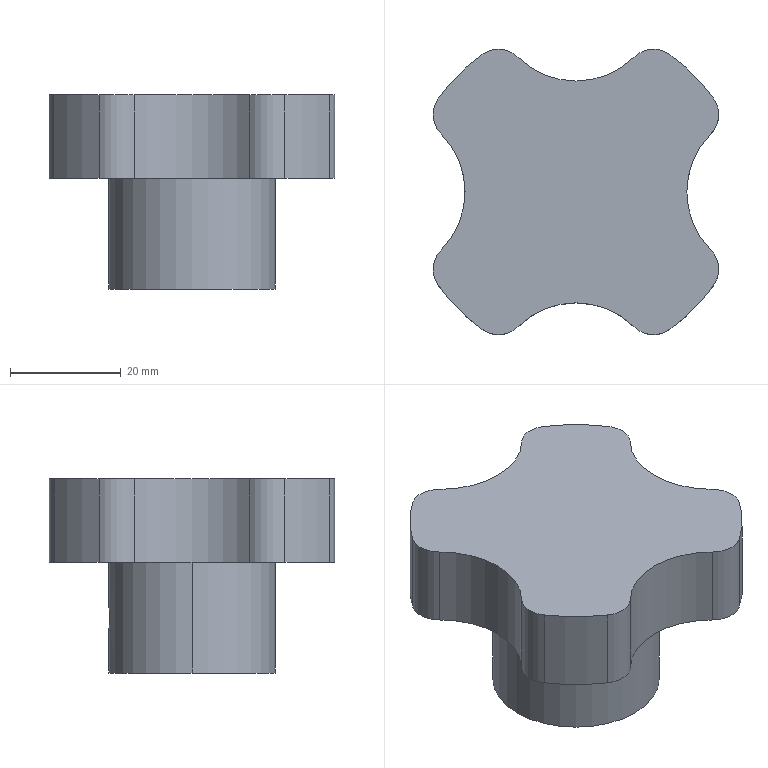Part | STEP file | Nylon handwheel sleeve QY-1-37 | 1 solid | 29 faces | box 51.477 x 51.477 x 35 mm | volume 42293 mm3 | cylinder 25 | plane 4 | commonest cylinder face diameters 10 x10 29.703 x5 60 x4 4.2 x2 14 x2 30 x2